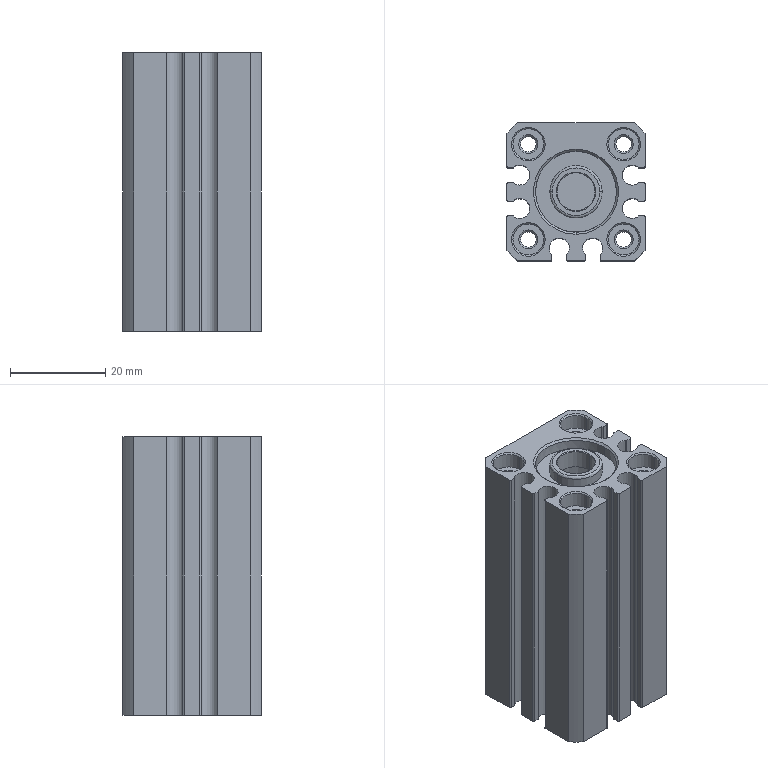Part | STEP file | HI_JSNR16X30_body_default | 1 solid | 170 faces | box 29 x 29 x 58.5 mm | volume 29020 mm3 | cylinder 72 | plane 52 | cone 42 | spline 4 | commonest cylinder face diameters 6.5 x16 0.6 x12 4.2 x12 3.242 x8 1.5 x4 4.134 x4